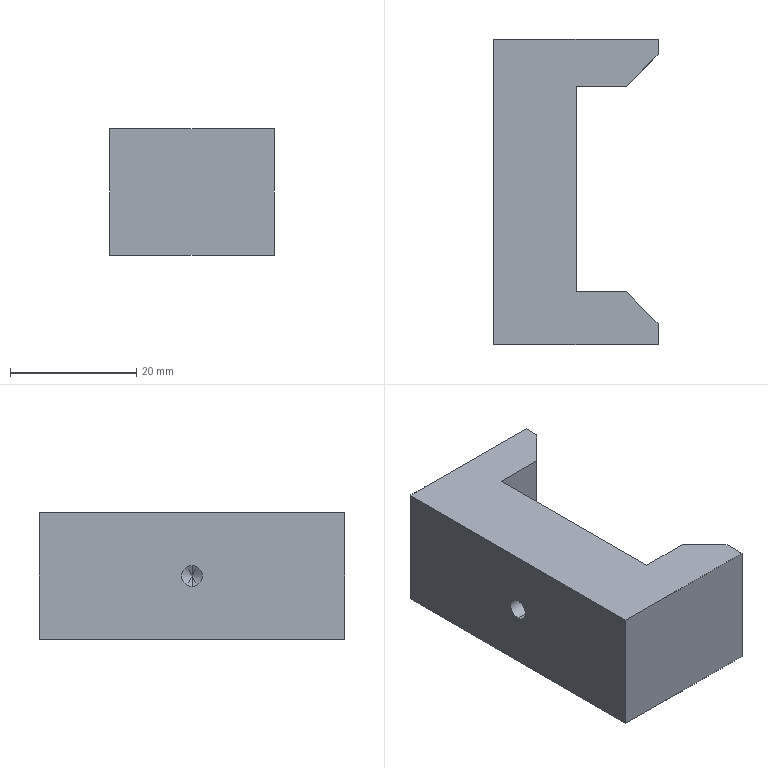Part | STEP file | 超声ProductFixed夹-2 | 1 solid | 16 faces | box 25.961 x 48.342 x 20 mm | volume 16055 mm3 | plane 12 | cylinder 2 | cone 2 | commonest cylinder face diameters 3.3 x2
STEP:
#1=CARTESIAN_POINT('',(-36.514,115.226,8.35));
#2=VERTEX_POINT('',#1);
#3=CARTESIAN_POINT('',(-36.514,115.226,11.65));
#4=VERTEX_POINT('',#3);
#5=CARTESIAN_POINT('',(-36.514,115.226,10.));
#6=DIRECTION('',(-1.,0.,0.));
#7=DIRECTION('',(0.,0.,1.));
#8=AXIS2_PLACEMENT_3D('',#5,#6,#7);
#9=CIRCLE('',#8,1.65);
#10=EDGE_CURVE('',#2,#4,#9,.T.);
#11=ORIENTED_EDGE('',*,*,#10,.F.);
#12=CARTESIAN_POINT('',(-48.014,115.226,8.35));
#13=VERTEX_POINT('',#12);
#14=CARTESIAN_POINT('',(-48.014,115.226,8.35));
#15=DIRECTION('',(-1.,0.,0.));
#16=VECTOR('',#15,1000.);
#17=LINE('',#14,#16);
#18=EDGE_CURVE('',#2,#13,#17,.T.);
#19=ORIENTED_EDGE('',*,*,#18,.T.);
#20=CARTESIAN_POINT('',(-48.014,115.226,11.65));
#21=VERTEX_POINT('',#20);
#22=CARTESIAN_POINT('',(-48.014,115.226,10.));
#23=DIRECTION('',(-1.,0.,0.));
#24=DIRECTION('',(0.,0.,1.));
#25=AXIS2_PLACEMENT_3D('',#22,#23,#24);
#26=CIRCLE('',#25,1.65);
#27=EDGE_CURVE('',#13,#21,#26,.T.);
#28=ORIENTED_EDGE('',*,*,#27,.T.);
#29=CARTESIAN_POINT('',(-48.014,115.226,11.65));
#30=DIRECTION('',(-1.,0.,0.));
#31=VECTOR('',#30,1000.);
#32=LINE('',#29,#31);
#33=EDGE_CURVE('',#4,#21,#32,.T.);
#34=ORIENTED_EDGE('',*,*,#33,.F.);
#35=EDGE_LOOP('',(#11,#19,#28,#34));
#36=FACE_OUTER_BOUND('',#35,.T.);
#37=CARTESIAN_POINT('',(-48.014,115.226,10.));
#38=DIRECTION('',(-1.,0.,0.));
#39=DIRECTION('',(0.,0.,1.));
#40=AXIS2_PLACEMENT_3D('',#37,#38,#39);
#41=CYLINDRICAL_SURFACE('',#40,1.65);
#42=ADVANCED_FACE('',(#36),#41,.F.);
#43=CARTESIAN_POINT('',(-35.523,115.226,10.));
#44=VERTEX_POINT('',#43);
#45=CARTESIAN_POINT('',(-36.514,115.226,11.65));
#46=DIRECTION('',(-0.515,0.,0.8572));
#47=VECTOR('',#46,1000.);
#48=LINE('',#45,#47);
#49=EDGE_CURVE('',#44,#4,#48,.T.);
#50=ORIENTED_EDGE('',*,*,#49,.F.);
#51=CARTESIAN_POINT('',(-36.514,115.226,8.35));
#52=DIRECTION('',(-0.515,0.,-0.8572));
#53=VECTOR('',#52,1000.);
#54=LINE('',#51,#53);
#55=EDGE_CURVE('',#44,#2,#54,.T.);
#56=ORIENTED_EDGE('',*,*,#55,.T.);
#57=ORIENTED_EDGE('',*,*,#10,.T.);
#58=EDGE_LOOP('',(#50,#56,#57));
#59=FACE_OUTER_BOUND('',#58,.T.);
#60=CARTESIAN_POINT('',(-36.514,115.226,10.));
#61=DIRECTION('',(-1.,0.,0.));
#62=DIRECTION('',(0.,0.,1.));
#63=AXIS2_PLACEMENT_3D('',#60,#61,#62);
#64=CONICAL_SURFACE('',#63,1.65,1.03);
#65=ADVANCED_FACE('',(#59),#64,.F.);
#66=CARTESIAN_POINT('',(-48.014,115.226,10.));
#67=DIRECTION('',(-1.,0.,0.));
#68=DIRECTION('',(0.,0.,1.));
#69=AXIS2_PLACEMENT_3D('',#66,#67,#68);
#70=CIRCLE('',#69,1.65);
#71=EDGE_CURVE('',#21,#13,#70,.T.);
#72=ORIENTED_EDGE('',*,*,#71,.F.);
#73=ORIENTED_EDGE('',*,*,#27,.F.);
#74=EDGE_LOOP('',(#72,#73));
#75=FACE_BOUND('',#74,.T.);
#76=CARTESIAN_POINT('',(-48.014,139.396,0.));
#77=VERTEX_POINT('',#76);
#78=CARTESIAN_POINT('',(-48.014,91.055,0.));
#79=VERTEX_POINT('',#78);
#80=CARTESIAN_POINT('',(-48.014,91.055,0.));
#81=DIRECTION('',(0.,-1.,0.));
#82=VECTOR('',#81,1000.);
#83=LINE('',#80,#82);
#84=EDGE_CURVE('',#77,#79,#83,.T.);
#85=ORIENTED_EDGE('',*,*,#84,.T.);
#86=CARTESIAN_POINT('',(-48.014,91.055,20.));
#87=VERTEX_POINT('',#86);
#88=CARTESIAN_POINT('',(-48.014,91.055,20.));
#89=DIRECTION('',(0.,0.,-1.));
#90=VECTOR('',#89,1000.);
#91=LINE('',#88,#90);
#92=EDGE_CURVE('',#87,#79,#91,.T.);
#93=ORIENTED_EDGE('',*,*,#92,.F.);
#94=CARTESIAN_POINT('',(-48.014,139.396,20.));
#95=VERTEX_POINT('',#94);
#96=CARTESIAN_POINT('',(-48.014,91.055,20.));
#97=DIRECTION('',(0.,-1.,0.));
#98=VECTOR('',#97,1000.);
#99=LINE('',#96,#98);
#100=EDGE_CURVE('',#95,#87,#99,.T.);
#101=ORIENTED_EDGE('',*,*,#100,.F.);
#102=CARTESIAN_POINT('',(-48.014,139.396,20.));
#103=DIRECTION('',(0.,0.,-1.));
#104=VECTOR('',#103,1000.);
#105=LINE('',#102,#104);
#106=EDGE_CURVE('',#95,#77,#105,.T.);
#107=ORIENTED_EDGE('',*,*,#106,.T.);
#108=EDGE_LOOP('',(#85,#93,#101,#107));
#109=FACE_OUTER_BOUND('',#108,.T.);
#110=CARTESIAN_POINT('',(-48.014,91.055,20.));
#111=DIRECTION('',(1.,0.,0.));
#112=DIRECTION('',(0.,0.,-1.));
#113=AXIS2_PLACEMENT_3D('',#110,#111,#112);
#114=PLANE('',#113);
#115=ADVANCED_FACE('',(#75,#109),#114,.F.);
#116=CARTESIAN_POINT('',(-22.053,91.055,0.));
#117=VERTEX_POINT('',#116);
#118=CARTESIAN_POINT('',(-48.014,91.055,0.));
#119=DIRECTION('',(1.,0.,0.));
#120=VECTOR('',#119,1000.);
#121=LINE('',#118,#120);
#122=EDGE_CURVE('',#79,#117,#121,.T.);
#123=ORIENTED_EDGE('',*,*,#122,.T.);
#124=CARTESIAN_POINT('',(-22.053,91.055,20.));
#125=VERTEX_POINT('',#124);
#126=CARTESIAN_POINT('',(-22.053,91.055,20.));
#127=DIRECTION('',(0.,0.,-1.));
#128=VECTOR('',#127,1000.);
#129=LINE('',#126,#128);
#130=EDGE_CURVE('',#125,#117,#129,.T.);
#131=ORIENTED_EDGE('',*,*,#130,.F.);
#132=CARTESIAN_POINT('',(-48.014,91.055,20.));
#133=DIRECTION('',(1.,0.,0.));
#134=VECTOR('',#133,1000.);
#135=LINE('',#132,#134);
#136=EDGE_CURVE('',#87,#125,#135,.T.);
#137=ORIENTED_EDGE('',*,*,#136,.F.);
#138=ORIENTED_EDGE('',*,*,#92,.T.);
#139=EDGE_LOOP('',(#123,#131,#137,#138));
#140=FACE_OUTER_BOUND('',#139,.T.);
#141=CARTESIAN_POINT('',(-48.014,91.055,20.));
#142=DIRECTION('',(0.,1.,0.));
#143=DIRECTION('',(0.,0.,1.));
#144=AXIS2_PLACEMENT_3D('',#141,#142,#143);
#145=PLANE('',#144);
#146=ADVANCED_FACE('',(#140),#145,.F.);
#147=CARTESIAN_POINT('',(-22.053,94.41,0.));
#148=VERTEX_POINT('',#147);
#149=CARTESIAN_POINT('',(-22.053,91.055,0.));
#150=DIRECTION('',(0.,1.,0.));
#151=VECTOR('',#150,1000.);
#152=LINE('',#149,#151);
#153=EDGE_CURVE('',#117,#148,#152,.T.);
#154=ORIENTED_EDGE('',*,*,#153,.T.);
#155=CARTESIAN_POINT('',(-22.053,94.41,20.));
#156=VERTEX_POINT('',#155);
#157=CARTESIAN_POINT('',(-22.053,94.41,20.));
#158=DIRECTION('',(0.,0.,-1.));
#159=VECTOR('',#158,1000.);
#160=LINE('',#157,#159);
#161=EDGE_CURVE('',#156,#148,#160,.T.);
#162=ORIENTED_EDGE('',*,*,#161,.F.);
#163=CARTESIAN_POINT('',(-22.053,91.055,20.));
#164=DIRECTION('',(0.,1.,0.));
#165=VECTOR('',#164,1000.);
#166=LINE('',#163,#165);
#167=EDGE_CURVE('',#125,#156,#166,.T.);
#168=ORIENTED_EDGE('',*,*,#167,.F.);
#169=ORIENTED_EDGE('',*,*,#130,.T.);
#170=EDGE_LOOP('',(#154,#162,#168,#169));
#171=FACE_OUTER_BOUND('',#170,.T.);
#172=CARTESIAN_POINT('',(-22.053,91.055,20.));
#173=DIRECTION('',(-1.,0.,0.));
#174=DIRECTION('',(0.,0.,1.));
#175=AXIS2_PLACEMENT_3D('',#172,#173,#174);
#176=PLANE('',#175);
#177=ADVANCED_FACE('',(#171),#176,.F.);
#178=CARTESIAN_POINT('',(-27.053,99.41,0.));
#179=VERTEX_POINT('',#178);
#180=CARTESIAN_POINT('',(-22.053,94.41,0.));
#181=DIRECTION('',(-0.7071,0.7071,0.));
#182=VECTOR('',#181,1000.);
#183=LINE('',#180,#182);
#184=EDGE_CURVE('',#148,#179,#183,.T.);
#185=ORIENTED_EDGE('',*,*,#184,.T.);
#186=CARTESIAN_POINT('',(-27.053,99.41,20.));
#187=VERTEX_POINT('',#186);
#188=CARTESIAN_POINT('',(-27.053,99.41,20.));
#189=DIRECTION('',(0.,0.,-1.));
#190=VECTOR('',#189,1000.);
#191=LINE('',#188,#190);
#192=EDGE_CURVE('',#187,#179,#191,.T.);
#193=ORIENTED_EDGE('',*,*,#192,.F.);
#194=CARTESIAN_POINT('',(-22.053,94.41,20.));
#195=DIRECTION('',(-0.7071,0.7071,0.));
#196=VECTOR('',#195,1000.);
#197=LINE('',#194,#196);
#198=EDGE_CURVE('',#156,#187,#197,.T.);
#199=ORIENTED_EDGE('',*,*,#198,.F.);
#200=ORIENTED_EDGE('',*,*,#161,.T.);
#201=EDGE_LOOP('',(#185,#193,#199,#200));
#202=FACE_OUTER_BOUND('',#201,.T.);
#203=CARTESIAN_POINT('',(-22.053,94.41,20.));
#204=DIRECTION('',(-0.7071,-0.7071,0.));
#205=DIRECTION('',(0.7071,-0.7071,0.));
#206=AXIS2_PLACEMENT_3D('',#203,#204,#205);
#207=PLANE('',#206);
#208=ADVANCED_FACE('',(#202),#207,.F.);
#209=CARTESIAN_POINT('',(-35.034,99.41,0.));
#210=VERTEX_POINT('',#209);
#211=CARTESIAN_POINT('',(-27.053,99.41,0.));
#212=DIRECTION('',(-1.,0.,0.));
#213=VECTOR('',#212,1000.);
#214=LINE('',#211,#213);
#215=EDGE_CURVE('',#179,#210,#214,.T.);
#216=ORIENTED_EDGE('',*,*,#215,.T.);
#217=CARTESIAN_POINT('',(-35.034,99.41,20.));
#218=VERTEX_POINT('',#217);
#219=CARTESIAN_POINT('',(-35.034,99.41,20.));
#220=DIRECTION('',(0.,0.,-1.));
#221=VECTOR('',#220,1000.);
#222=LINE('',#219,#221);
#223=EDGE_CURVE('',#218,#210,#222,.T.);
#224=ORIENTED_EDGE('',*,*,#223,.F.);
#225=CARTESIAN_POINT('',(-27.053,99.41,20.));
#226=DIRECTION('',(-1.,0.,0.));
#227=VECTOR('',#226,1000.);
#228=LINE('',#225,#227);
#229=EDGE_CURVE('',#187,#218,#228,.T.);
#230=ORIENTED_EDGE('',*,*,#229,.F.);
#231=ORIENTED_EDGE('',*,*,#192,.T.);
#232=EDGE_LOOP('',(#216,#224,#230,#231));
#233=FACE_OUTER_BOUND('',#232,.T.);
#234=CARTESIAN_POINT('',(-27.053,99.41,20.));
#235=DIRECTION('',(0.,-1.,0.));
#236=DIRECTION('',(0.,0.,-1.));
#237=AXIS2_PLACEMENT_3D('',#234,#235,#236);
#238=PLANE('',#237);
#239=ADVANCED_FACE('',(#233),#238,.F.);
#240=CARTESIAN_POINT('',(-35.034,131.936,0.));
#241=VERTEX_POINT('',#240);
#242=CARTESIAN_POINT('',(-35.034,131.936,0.));
#243=DIRECTION('',(0.,1.,0.));
#244=VECTOR('',#243,1000.);
#245=LINE('',#242,#244);
#246=EDGE_CURVE('',#210,#241,#245,.T.);
#247=ORIENTED_EDGE('',*,*,#246,.T.);
#248=CARTESIAN_POINT('',(-35.034,131.936,20.));
#249=VERTEX_POINT('',#248);
#250=CARTESIAN_POINT('',(-35.034,131.936,20.));
#251=DIRECTION('',(0.,0.,-1.));
#252=VECTOR('',#251,1000.);
#253=LINE('',#250,#252);
#254=EDGE_CURVE('',#249,#241,#253,.T.);
#255=ORIENTED_EDGE('',*,*,#254,.F.);
#256=CARTESIAN_POINT('',(-35.034,131.936,20.));
#257=DIRECTION('',(0.,1.,0.));
#258=VECTOR('',#257,1000.);
#259=LINE('',#256,#258);
#260=EDGE_CURVE('',#218,#249,#259,.T.);
#261=ORIENTED_EDGE('',*,*,#260,.F.);
#262=ORIENTED_EDGE('',*,*,#223,.T.);
#263=EDGE_LOOP('',(#247,#255,#261,#262));
#264=FACE_OUTER_BOUND('',#263,.T.);
#265=CARTESIAN_POINT('',(-35.034,131.936,20.));
#266=DIRECTION('',(-1.,0.,0.));
#267=DIRECTION('',(0.,0.,1.));
#268=AXIS2_PLACEMENT_3D('',#265,#266,#267);
#269=PLANE('',#268);
#270=ADVANCED_FACE('',(#264),#269,.F.);
#271=CARTESIAN_POINT('',(-27.053,131.936,0.));
#272=VERTEX_POINT('',#271);
#273=CARTESIAN_POINT('',(-27.053,131.936,0.));
#274=DIRECTION('',(1.,0.,0.));
#275=VECTOR('',#274,1000.);
#276=LINE('',#273,#275);
#277=EDGE_CURVE('',#241,#272,#276,.T.);
#278=ORIENTED_EDGE('',*,*,#277,.T.);
#279=CARTESIAN_POINT('',(-27.053,131.936,20.));
#280=VERTEX_POINT('',#279);
#281=CARTESIAN_POINT('',(-27.053,131.936,20.));
#282=DIRECTION('',(0.,0.,-1.));
#283=VECTOR('',#282,1000.);
#284=LINE('',#281,#283);
#285=EDGE_CURVE('',#280,#272,#284,.T.);
#286=ORIENTED_EDGE('',*,*,#285,.F.);
#287=CARTESIAN_POINT('',(-27.053,131.936,20.));
#288=DIRECTION('',(1.,0.,0.));
#289=VECTOR('',#288,1000.);
#290=LINE('',#287,#289);
#291=EDGE_CURVE('',#249,#280,#290,.T.);
#292=ORIENTED_EDGE('',*,*,#291,.F.);
#293=ORIENTED_EDGE('',*,*,#254,.T.);
#294=EDGE_LOOP('',(#278,#286,#292,#293));
#295=FACE_OUTER_BOUND('',#294,.T.);
#296=CARTESIAN_POINT('',(-27.053,131.936,20.));
#297=DIRECTION('',(0.,1.,0.));
#298=DIRECTION('',(0.,0.,1.));
#299=AXIS2_PLACEMENT_3D('',#296,#297,#298);
#300=PLANE('',#299);
#301=ADVANCED_FACE('',(#295),#300,.F.);
#302=CARTESIAN_POINT('',(-22.053,136.936,0.));
#303=VERTEX_POINT('',#302);
#304=CARTESIAN_POINT('',(-27.053,131.936,0.));
#305=DIRECTION('',(0.7071,0.7071,0.));
#306=VECTOR('',#305,1000.);
#307=LINE('',#304,#306);
#308=EDGE_CURVE('',#272,#303,#307,.T.);
#309=ORIENTED_EDGE('',*,*,#308,.T.);
#310=CARTESIAN_POINT('',(-22.053,136.936,20.));
#311=VERTEX_POINT('',#310);
#312=CARTESIAN_POINT('',(-22.053,136.936,20.));
#313=DIRECTION('',(0.,0.,-1.));
#314=VECTOR('',#313,1000.);
#315=LINE('',#312,#314);
#316=EDGE_CURVE('',#311,#303,#315,.T.);
#317=ORIENTED_EDGE('',*,*,#316,.F.);
#318=CARTESIAN_POINT('',(-27.053,131.936,20.));
#319=DIRECTION('',(0.7071,0.7071,0.));
#320=VECTOR('',#319,1000.);
#321=LINE('',#318,#320);
#322=EDGE_CURVE('',#280,#311,#321,.T.);
#323=ORIENTED_EDGE('',*,*,#322,.F.);
#324=ORIENTED_EDGE('',*,*,#285,.T.);
#325=EDGE_LOOP('',(#309,#317,#323,#324));
#326=FACE_OUTER_BOUND('',#325,.T.);
#327=CARTESIAN_POINT('',(-27.053,131.936,20.));
#328=DIRECTION('',(-0.7071,0.7071,0.));
#329=DIRECTION('',(-0.7071,-0.7071,0.));
#330=AXIS2_PLACEMENT_3D('',#327,#328,#329);
#331=PLANE('',#330);
#332=ADVANCED_FACE('',(#326),#331,.F.);
#333=CARTESIAN_POINT('',(-22.053,139.396,0.));
#334=VERTEX_POINT('',#333);
#335=CARTESIAN_POINT('',(-22.053,136.936,0.));
#336=DIRECTION('',(0.,1.,0.));
#337=VECTOR('',#336,1000.);
#338=LINE('',#335,#337);
#339=EDGE_CURVE('',#303,#334,#338,.T.);
#340=ORIENTED_EDGE('',*,*,#339,.T.);
#341=CARTESIAN_POINT('',(-22.053,139.396,20.));
#342=VERTEX_POINT('',#341);
#343=CARTESIAN_POINT('',(-22.053,139.396,20.));
#344=DIRECTION('',(0.,0.,-1.));
#345=VECTOR('',#344,1000.);
#346=LINE('',#343,#345);
#347=EDGE_CURVE('',#342,#334,#346,.T.);
#348=ORIENTED_EDGE('',*,*,#347,.F.);
#349=CARTESIAN_POINT('',(-22.053,136.936,20.));
#350=DIRECTION('',(0.,1.,0.));
#351=VECTOR('',#350,1000.);
#352=LINE('',#349,#351);
#353=EDGE_CURVE('',#311,#342,#352,.T.);
#354=ORIENTED_EDGE('',*,*,#353,.F.);
#355=ORIENTED_EDGE('',*,*,#316,.T.);
#356=EDGE_LOOP('',(#340,#348,#354,#355));
#357=FACE_OUTER_BOUND('',#356,.T.);
#358=CARTESIAN_POINT('',(-22.053,136.936,20.));
#359=DIRECTION('',(-1.,0.,0.));
#360=DIRECTION('',(0.,0.,1.));
#361=AXIS2_PLACEMENT_3D('',#358,#359,#360);
#362=PLANE('',#361);
#363=ADVANCED_FACE('',(#357),#362,.F.);
#364=CARTESIAN_POINT('',(-48.014,139.396,0.));
#365=DIRECTION('',(-1.,0.,0.));
#366=VECTOR('',#365,1000.);
#367=LINE('',#364,#366);
#368=EDGE_CURVE('',#334,#77,#367,.T.);
#369=ORIENTED_EDGE('',*,*,#368,.T.);
#370=ORIENTED_EDGE('',*,*,#106,.F.);
#371=CARTESIAN_POINT('',(-48.014,139.396,20.));
#372=DIRECTION('',(-1.,0.,0.));
#373=VECTOR('',#372,1000.);
#374=LINE('',#371,#373);
#375=EDGE_CURVE('',#342,#95,#374,.T.);
#376=ORIENTED_EDGE('',*,*,#375,.F.);
#377=ORIENTED_EDGE('',*,*,#347,.T.);
#378=EDGE_LOOP('',(#369,#370,#376,#377));
#379=FACE_OUTER_BOUND('',#378,.T.);
#380=CARTESIAN_POINT('',(-48.014,139.396,20.));
#381=DIRECTION('',(0.,-1.,0.));
#382=DIRECTION('',(0.,0.,-1.));
#383=AXIS2_PLACEMENT_3D('',#380,#381,#382);
#384=PLANE('',#383);
#385=ADVANCED_FACE('',(#379),#384,.F.);
#386=ORIENTED_EDGE('',*,*,#100,.T.);
#387=ORIENTED_EDGE('',*,*,#136,.T.);
#388=ORIENTED_EDGE('',*,*,#167,.T.);
#389=ORIENTED_EDGE('',*,*,#198,.T.);
#390=ORIENTED_EDGE('',*,*,#229,.T.);
#391=ORIENTED_EDGE('',*,*,#260,.T.);
#392=ORIENTED_EDGE('',*,*,#291,.T.);
#393=ORIENTED_EDGE('',*,*,#322,.T.);
#394=ORIENTED_EDGE('',*,*,#353,.T.);
#395=ORIENTED_EDGE('',*,*,#375,.T.);
#396=EDGE_LOOP('',(#386,#387,#388,#389,#390,#391,#392,#393,#394,#395));
#397=FACE_OUTER_BOUND('',#396,.T.);
#398=CARTESIAN_POINT('',(-48.014,139.396,20.));
#399=DIRECTION('',(0.,0.,-1.));
#400=DIRECTION('',(-1.,0.,0.));
#401=AXIS2_PLACEMENT_3D('',#398,#399,#400);
#402=PLANE('',#401);
#403=ADVANCED_FACE('',(#397),#402,.F.);
#404=ORIENTED_EDGE('',*,*,#84,.F.);
#405=ORIENTED_EDGE('',*,*,#368,.F.);
#406=ORIENTED_EDGE('',*,*,#339,.F.);
#407=ORIENTED_EDGE('',*,*,#308,.F.);
#408=ORIENTED_EDGE('',*,*,#277,.F.);
#409=ORIENTED_EDGE('',*,*,#246,.F.);
#410=ORIENTED_EDGE('',*,*,#215,.F.);
#411=ORIENTED_EDGE('',*,*,#184,.F.);
#412=ORIENTED_EDGE('',*,*,#153,.F.);
#413=ORIENTED_EDGE('',*,*,#122,.F.);
#414=EDGE_LOOP('',(#404,#405,#406,#407,#408,#409,#410,#411,#412,#413));
#415=FACE_OUTER_BOUND('',#414,.T.);
#416=CARTESIAN_POINT('',(-48.014,139.396,0.));
#417=DIRECTION('',(0.,0.,-1.));
#418=DIRECTION('',(-1.,0.,0.));
#419=AXIS2_PLACEMENT_3D('',#416,#417,#418);
#420=PLANE('',#419);
#421=ADVANCED_FACE('',(#415),#420,.T.);
#422=ORIENTED_EDGE('',*,*,#55,.F.);
#423=ORIENTED_EDGE('',*,*,#49,.T.);
#424=CARTESIAN_POINT('',(-36.514,115.226,10.));
#425=DIRECTION('',(-1.,0.,0.));
#426=DIRECTION('',(0.,0.,1.));
#427=AXIS2_PLACEMENT_3D('',#424,#425,#426);
#428=CIRCLE('',#427,1.65);
#429=EDGE_CURVE('',#4,#2,#428,.T.);
#430=ORIENTED_EDGE('',*,*,#429,.T.);
#431=EDGE_LOOP('',(#422,#423,#430));
#432=FACE_OUTER_BOUND('',#431,.T.);
#433=CARTESIAN_POINT('',(-36.514,115.226,10.));
#434=DIRECTION('',(-1.,0.,0.));
#435=DIRECTION('',(0.,0.,1.));
#436=AXIS2_PLACEMENT_3D('',#433,#434,#435);
#437=CONICAL_SURFACE('',#436,1.65,1.03);
#438=ADVANCED_FACE('',(#432),#437,.F.);
#439=ORIENTED_EDGE('',*,*,#18,.F.);
#440=ORIENTED_EDGE('',*,*,#429,.F.);
#441=ORIENTED_EDGE('',*,*,#33,.T.);
#442=ORIENTED_EDGE('',*,*,#71,.T.);
#443=EDGE_LOOP('',(#439,#440,#441,#442));
#444=FACE_OUTER_BOUND('',#443,.T.);
#445=CARTESIAN_POINT('',(-48.014,115.226,10.));
#446=DIRECTION('',(-1.,0.,0.));
#447=DIRECTION('',(0.,0.,1.));
#448=AXIS2_PLACEMENT_3D('',#445,#446,#447);
#449=CYLINDRICAL_SURFACE('',#448,1.65);
#450=ADVANCED_FACE('',(#444),#449,.F.);
#451=CLOSED_SHELL('',(#42,#65,#115,#146,#177,#208,#239,#270,#301,#332,#363,#385,#403,#421,#438,#450));
#452=MANIFOLD_SOLID_BREP('',#451);
#453=CARTESIAN_POINT('',(0.,0.,0.));
#454=DIRECTION('',(0.,0.,1.));
#455=DIRECTION('',(1.,0.,0.));
#456=AXIS2_PLACEMENT_3D('',#453,#454,#455);
#457=(LENGTH_UNIT()NAMED_UNIT(*)SI_UNIT(.MILLI.,.METRE.));
#458=UNCERTAINTY_MEASURE_WITH_UNIT(LENGTH_MEASURE(0.00001),#457,'','');
#459=(NAMED_UNIT(*)PLANE_ANGLE_UNIT()SI_UNIT($,.RADIAN.));
#460=(NAMED_UNIT(*)SI_UNIT($,.STERADIAN.)SOLID_ANGLE_UNIT());
#461=(GEOMETRIC_REPRESENTATION_CONTEXT(3)GLOBAL_UNCERTAINTY_ASSIGNED_CONTEXT((#458))GLOBAL_UNIT_ASSIGNED_CONTEXT((#457,#459,#460))REPRESENTATION_CONTEXT('',''));
#462=ADVANCED_BREP_SHAPE_REPRESENTATION('',(#452,#456),#461);